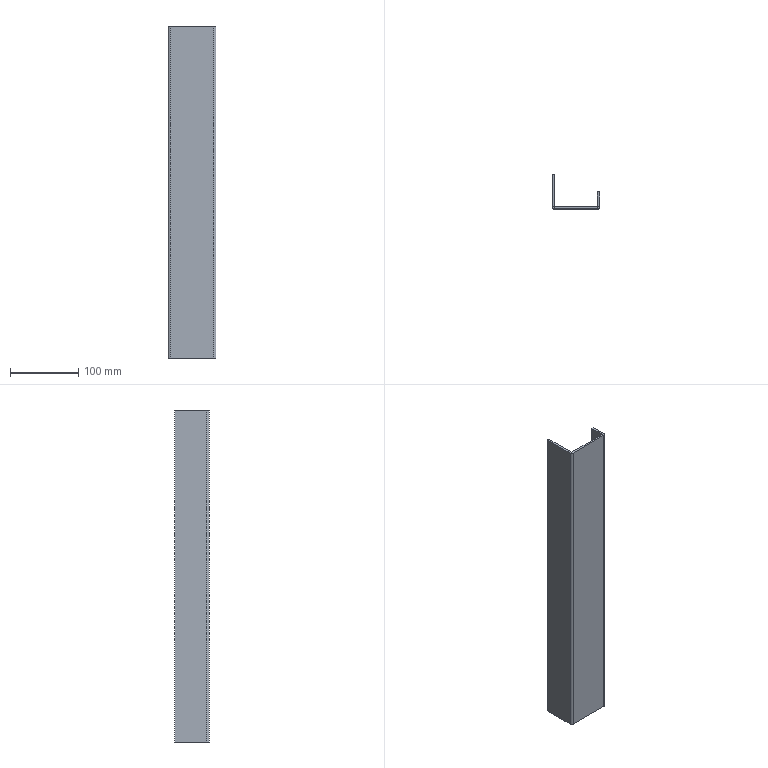Part | SolidWorks | 1 solid | 22 faces | box 69.995 x 50 x 485 mm | volume 200160 mm3 | plane 18 | cylinder 4 | commonest cylinder face diameters 0.2 x2 6.2 x2
STEP:
#1=CARTESIAN_POINT('',(31.895,-3.,-242.5));
#2=VERTEX_POINT('',#1);
#3=CARTESIAN_POINT('',(31.895,-3.,242.5));
#4=VERTEX_POINT('',#3);
#5=CARTESIAN_POINT('',(31.895,-3.,-242.5));
#6=DIRECTION('',(0.,0.,1.));
#7=VECTOR('',#6,1000.);
#8=LINE('',#5,#7);
#9=EDGE_CURVE('',#2,#4,#8,.T.);
#10=ORIENTED_EDGE('',*,*,#9,.T.);
#11=CARTESIAN_POINT('',(-31.9,-3.,242.5));
#12=VERTEX_POINT('',#11);
#13=CARTESIAN_POINT('',(35.,-3.,242.5));
#14=DIRECTION('',(1.,0.,0.));
#15=VECTOR('',#14,1000.);
#16=LINE('',#13,#15);
#17=EDGE_CURVE('',#12,#4,#16,.T.);
#18=ORIENTED_EDGE('',*,*,#17,.F.);
#19=CARTESIAN_POINT('',(-31.9,-3.,-242.5));
#20=VERTEX_POINT('',#19);
#21=CARTESIAN_POINT('',(-31.9,-3.,242.5));
#22=DIRECTION('',(0.,0.,-1.));
#23=VECTOR('',#22,1000.);
#24=LINE('',#21,#23);
#25=EDGE_CURVE('',#12,#20,#24,.T.);
#26=ORIENTED_EDGE('',*,*,#25,.T.);
#27=CARTESIAN_POINT('',(35.,-3.,-242.5));
#28=DIRECTION('',(-1.,0.,0.));
#29=VECTOR('',#28,1000.);
#30=LINE('',#27,#29);
#31=EDGE_CURVE('',#2,#20,#30,.T.);
#32=ORIENTED_EDGE('',*,*,#31,.F.);
#33=EDGE_LOOP('',(#10,#18,#26,#32));
#34=FACE_OUTER_BOUND('',#33,.T.);
#35=CARTESIAN_POINT('',(0.,-3.,0.));
#36=DIRECTION('',(0.,1.,0.));
#37=DIRECTION('',(0.,0.,1.));
#38=AXIS2_PLACEMENT_3D('',#35,#36,#37);
#39=PLANE('',#38);
#40=ADVANCED_FACE('',(#34),#39,.F.);
#41=CARTESIAN_POINT('',(-31.9,0.,242.5));
#42=VERTEX_POINT('',#41);
#43=CARTESIAN_POINT('',(31.895,0.,242.5));
#44=VERTEX_POINT('',#43);
#45=CARTESIAN_POINT('',(35.,0.,242.5));
#46=DIRECTION('',(1.,0.,0.));
#47=VECTOR('',#46,1000.);
#48=LINE('',#45,#47);
#49=EDGE_CURVE('',#42,#44,#48,.T.);
#50=ORIENTED_EDGE('',*,*,#49,.T.);
#51=CARTESIAN_POINT('',(31.895,0.,-242.5));
#52=VERTEX_POINT('',#51);
#53=CARTESIAN_POINT('',(31.895,0.,-242.5));
#54=DIRECTION('',(0.,0.,1.));
#55=VECTOR('',#54,1000.);
#56=LINE('',#53,#55);
#57=EDGE_CURVE('',#52,#44,#56,.T.);
#58=ORIENTED_EDGE('',*,*,#57,.F.);
#59=CARTESIAN_POINT('',(-31.9,0.,-242.5));
#60=VERTEX_POINT('',#59);
#61=CARTESIAN_POINT('',(35.,0.,-242.5));
#62=DIRECTION('',(-1.,0.,0.));
#63=VECTOR('',#62,1000.);
#64=LINE('',#61,#63);
#65=EDGE_CURVE('',#52,#60,#64,.T.);
#66=ORIENTED_EDGE('',*,*,#65,.T.);
#67=CARTESIAN_POINT('',(-31.9,0.,242.5));
#68=DIRECTION('',(0.,0.,-1.));
#69=VECTOR('',#68,1000.);
#70=LINE('',#67,#69);
#71=EDGE_CURVE('',#42,#60,#70,.T.);
#72=ORIENTED_EDGE('',*,*,#71,.F.);
#73=EDGE_LOOP('',(#50,#58,#66,#72));
#74=FACE_OUTER_BOUND('',#73,.T.);
#75=CARTESIAN_POINT('',(0.,0.,0.));
#76=DIRECTION('',(0.,1.,0.));
#77=DIRECTION('',(0.,0.,1.));
#78=AXIS2_PLACEMENT_3D('',#75,#76,#77);
#79=PLANE('',#78);
#80=ADVANCED_FACE('',(#74),#79,.T.);
#81=ORIENTED_EDGE('',*,*,#65,.F.);
#82=CARTESIAN_POINT('',(31.895,0.,-242.5));
#83=DIRECTION('',(0.,-1.,0.));
#84=VECTOR('',#83,1000.);
#85=LINE('',#82,#84);
#86=EDGE_CURVE('',#52,#2,#85,.T.);
#87=ORIENTED_EDGE('',*,*,#86,.T.);
#88=ORIENTED_EDGE('',*,*,#31,.T.);
#89=CARTESIAN_POINT('',(-31.9,0.,-242.5));
#90=DIRECTION('',(0.,-1.,0.));
#91=VECTOR('',#90,1000.);
#92=LINE('',#89,#91);
#93=EDGE_CURVE('',#60,#20,#92,.T.);
#94=ORIENTED_EDGE('',*,*,#93,.F.);
#95=EDGE_LOOP('',(#81,#87,#88,#94));
#96=FACE_OUTER_BOUND('',#95,.T.);
#97=CARTESIAN_POINT('',(35.,-3.,-242.5));
#98=DIRECTION('',(0.,0.,-1.));
#99=DIRECTION('',(-1.,0.,0.));
#100=AXIS2_PLACEMENT_3D('',#97,#98,#99);
#101=PLANE('',#100);
#102=ADVANCED_FACE('',(#96),#101,.T.);
#103=CARTESIAN_POINT('',(31.895,0.,242.5));
#104=DIRECTION('',(0.,-1.,0.));
#105=VECTOR('',#104,1000.);
#106=LINE('',#103,#105);
#107=EDGE_CURVE('',#44,#4,#106,.T.);
#108=ORIENTED_EDGE('',*,*,#107,.F.);
#109=ORIENTED_EDGE('',*,*,#49,.F.);
#110=CARTESIAN_POINT('',(-31.9,0.,242.5));
#111=DIRECTION('',(0.,-1.,0.));
#112=VECTOR('',#111,1000.);
#113=LINE('',#110,#112);
#114=EDGE_CURVE('',#42,#12,#113,.T.);
#115=ORIENTED_EDGE('',*,*,#114,.T.);
#116=ORIENTED_EDGE('',*,*,#17,.T.);
#117=EDGE_LOOP('',(#108,#109,#115,#116));
#118=FACE_OUTER_BOUND('',#117,.T.);
#119=CARTESIAN_POINT('',(35.,-3.,242.5));
#120=DIRECTION('',(0.,0.,1.));
#121=DIRECTION('',(1.,0.,0.));
#122=AXIS2_PLACEMENT_3D('',#119,#120,#121);
#123=PLANE('',#122);
#124=ADVANCED_FACE('',(#118),#123,.T.);
#125=CARTESIAN_POINT('',(-32.,0.1,-242.5));
#126=VERTEX_POINT('',#125);
#127=CARTESIAN_POINT('',(-35.,0.1,-242.5));
#128=VERTEX_POINT('',#127);
#129=CARTESIAN_POINT('',(-35.,0.1,-242.5));
#130=DIRECTION('',(-1.,0.,0.));
#131=VECTOR('',#130,1000.);
#132=LINE('',#129,#131);
#133=EDGE_CURVE('',#126,#128,#132,.T.);
#134=ORIENTED_EDGE('',*,*,#133,.F.);
#135=CARTESIAN_POINT('',(-31.9,0.1,-242.5));
#136=DIRECTION('',(0.,0.,-1.));
#137=DIRECTION('',(1.,0.,0.));
#138=AXIS2_PLACEMENT_3D('',#135,#136,#137);
#139=CIRCLE('',#138,0.1);
#140=EDGE_CURVE('',#60,#126,#139,.T.);
#141=ORIENTED_EDGE('',*,*,#140,.F.);
#142=ORIENTED_EDGE('',*,*,#93,.T.);
#143=CARTESIAN_POINT('',(-31.9,0.1,-242.5));
#144=DIRECTION('',(0.,0.,-1.));
#145=DIRECTION('',(1.,0.,0.));
#146=AXIS2_PLACEMENT_3D('',#143,#144,#145);
#147=CIRCLE('',#146,3.1);
#148=EDGE_CURVE('',#20,#128,#147,.T.);
#149=ORIENTED_EDGE('',*,*,#148,.T.);
#150=EDGE_LOOP('',(#134,#141,#142,#149));
#151=FACE_OUTER_BOUND('',#150,.T.);
#152=CARTESIAN_POINT('',(-31.9,0.1,-242.5));
#153=DIRECTION('',(0.,0.,-1.));
#154=DIRECTION('',(-1.,0.,0.));
#155=AXIS2_PLACEMENT_3D('',#152,#153,#154);
#156=PLANE('',#155);
#157=ADVANCED_FACE('',(#151),#156,.T.);
#158=CARTESIAN_POINT('',(-32.,0.1,242.5));
#159=VERTEX_POINT('',#158);
#160=CARTESIAN_POINT('',(-31.9,0.1,242.5));
#161=DIRECTION('',(0.,0.,1.));
#162=DIRECTION('',(1.,0.,0.));
#163=AXIS2_PLACEMENT_3D('',#160,#161,#162);
#164=CIRCLE('',#163,0.1);
#165=EDGE_CURVE('',#159,#42,#164,.T.);
#166=ORIENTED_EDGE('',*,*,#165,.F.);
#167=CARTESIAN_POINT('',(-35.,0.1,242.5));
#168=VERTEX_POINT('',#167);
#169=CARTESIAN_POINT('',(-32.,0.1,242.5));
#170=DIRECTION('',(-1.,0.,0.));
#171=VECTOR('',#170,1000.);
#172=LINE('',#169,#171);
#173=EDGE_CURVE('',#159,#168,#172,.T.);
#174=ORIENTED_EDGE('',*,*,#173,.T.);
#175=CARTESIAN_POINT('',(-31.9,0.1,242.5));
#176=DIRECTION('',(0.,0.,1.));
#177=DIRECTION('',(1.,0.,0.));
#178=AXIS2_PLACEMENT_3D('',#175,#176,#177);
#179=CIRCLE('',#178,3.1);
#180=EDGE_CURVE('',#168,#12,#179,.T.);
#181=ORIENTED_EDGE('',*,*,#180,.T.);
#182=ORIENTED_EDGE('',*,*,#114,.F.);
#183=EDGE_LOOP('',(#166,#174,#181,#182));
#184=FACE_OUTER_BOUND('',#183,.T.);
#185=CARTESIAN_POINT('',(-31.9,0.1,242.5));
#186=DIRECTION('',(0.,0.,-1.));
#187=DIRECTION('',(-1.,0.,0.));
#188=AXIS2_PLACEMENT_3D('',#185,#186,#187);
#189=PLANE('',#188);
#190=ADVANCED_FACE('',(#184),#189,.F.);
#191=ORIENTED_EDGE('',*,*,#25,.F.);
#192=ORIENTED_EDGE('',*,*,#180,.F.);
#193=CARTESIAN_POINT('',(-35.,0.1,-242.5));
#194=DIRECTION('',(0.,0.,-1.));
#195=VECTOR('',#194,1000.);
#196=LINE('',#193,#195);
#197=EDGE_CURVE('',#168,#128,#196,.T.);
#198=ORIENTED_EDGE('',*,*,#197,.T.);
#199=ORIENTED_EDGE('',*,*,#148,.F.);
#200=EDGE_LOOP('',(#191,#192,#198,#199));
#201=FACE_OUTER_BOUND('',#200,.T.);
#202=CARTESIAN_POINT('',(-31.9,0.1,242.5));
#203=DIRECTION('',(0.,0.,1.));
#204=DIRECTION('',(-1.,0.,0.));
#205=AXIS2_PLACEMENT_3D('',#202,#203,#204);
#206=CYLINDRICAL_SURFACE('',#205,3.1);
#207=ADVANCED_FACE('',(#201),#206,.T.);
#208=ORIENTED_EDGE('',*,*,#71,.T.);
#209=ORIENTED_EDGE('',*,*,#140,.T.);
#210=CARTESIAN_POINT('',(-32.,0.1,-242.5));
#211=DIRECTION('',(0.,0.,1.));
#212=VECTOR('',#211,1000.);
#213=LINE('',#210,#212);
#214=EDGE_CURVE('',#126,#159,#213,.T.);
#215=ORIENTED_EDGE('',*,*,#214,.T.);
#216=ORIENTED_EDGE('',*,*,#165,.T.);
#217=EDGE_LOOP('',(#208,#209,#215,#216));
#218=FACE_OUTER_BOUND('',#217,.T.);
#219=CARTESIAN_POINT('',(-31.9,0.1,242.5));
#220=DIRECTION('',(0.,0.,1.));
#221=DIRECTION('',(-1.,0.,0.));
#222=AXIS2_PLACEMENT_3D('',#219,#220,#221);
#223=CYLINDRICAL_SURFACE('',#222,0.1);
#224=ADVANCED_FACE('',(#218),#223,.F.);
#225=ORIENTED_EDGE('',*,*,#133,.T.);
#226=CARTESIAN_POINT('',(-35.,47.,-242.5));
#227=VERTEX_POINT('',#226);
#228=CARTESIAN_POINT('',(-35.,0.,-242.5));
#229=DIRECTION('',(0.,-1.,0.));
#230=VECTOR('',#229,1000.);
#231=LINE('',#228,#230);
#232=EDGE_CURVE('',#227,#128,#231,.T.);
#233=ORIENTED_EDGE('',*,*,#232,.F.);
#234=CARTESIAN_POINT('',(-32.,47.,-242.5));
#235=VERTEX_POINT('',#234);
#236=CARTESIAN_POINT('',(-35.,47.,-242.5));
#237=DIRECTION('',(1.,0.,0.));
#238=VECTOR('',#237,1000.);
#239=LINE('',#236,#238);
#240=EDGE_CURVE('',#227,#235,#239,.T.);
#241=ORIENTED_EDGE('',*,*,#240,.T.);
#242=CARTESIAN_POINT('',(-32.,0.,-242.5));
#243=DIRECTION('',(0.,-1.,0.));
#244=VECTOR('',#243,1000.);
#245=LINE('',#242,#244);
#246=EDGE_CURVE('',#235,#126,#245,.T.);
#247=ORIENTED_EDGE('',*,*,#246,.T.);
#248=EDGE_LOOP('',(#225,#233,#241,#247));
#249=FACE_OUTER_BOUND('',#248,.T.);
#250=CARTESIAN_POINT('',(-35.,0.,-242.5));
#251=DIRECTION('',(0.,0.,1.));
#252=DIRECTION('',(1.,0.,0.));
#253=AXIS2_PLACEMENT_3D('',#250,#251,#252);
#254=PLANE('',#253);
#255=ADVANCED_FACE('',(#249),#254,.F.);
#256=ORIENTED_EDGE('',*,*,#173,.F.);
#257=CARTESIAN_POINT('',(-32.,47.,242.5));
#258=VERTEX_POINT('',#257);
#259=CARTESIAN_POINT('',(-32.,47.,242.5));
#260=DIRECTION('',(0.,1.,0.));
#261=VECTOR('',#260,1000.);
#262=LINE('',#259,#261);
#263=EDGE_CURVE('',#159,#258,#262,.T.);
#264=ORIENTED_EDGE('',*,*,#263,.T.);
#265=CARTESIAN_POINT('',(-35.,47.,242.5));
#266=VERTEX_POINT('',#265);
#267=CARTESIAN_POINT('',(-35.,47.,242.5));
#268=DIRECTION('',(1.,0.,0.));
#269=VECTOR('',#268,1000.);
#270=LINE('',#267,#269);
#271=EDGE_CURVE('',#266,#258,#270,.T.);
#272=ORIENTED_EDGE('',*,*,#271,.F.);
#273=CARTESIAN_POINT('',(-35.,0.,242.5));
#274=DIRECTION('',(0.,1.,0.));
#275=VECTOR('',#274,1000.);
#276=LINE('',#273,#275);
#277=EDGE_CURVE('',#168,#266,#276,.T.);
#278=ORIENTED_EDGE('',*,*,#277,.F.);
#279=EDGE_LOOP('',(#256,#264,#272,#278));
#280=FACE_OUTER_BOUND('',#279,.T.);
#281=CARTESIAN_POINT('',(-35.,47.,242.5));
#282=DIRECTION('',(0.,0.,-1.));
#283=DIRECTION('',(-1.,0.,0.));
#284=AXIS2_PLACEMENT_3D('',#281,#282,#283);
#285=PLANE('',#284);
#286=ADVANCED_FACE('',(#280),#285,.F.);
#287=ORIENTED_EDGE('',*,*,#197,.F.);
#288=ORIENTED_EDGE('',*,*,#277,.T.);
#289=CARTESIAN_POINT('',(-35.,47.,0.));
#290=DIRECTION('',(0.,0.,-1.));
#291=VECTOR('',#290,1000.);
#292=LINE('',#289,#291);
#293=EDGE_CURVE('',#266,#227,#292,.T.);
#294=ORIENTED_EDGE('',*,*,#293,.T.);
#295=ORIENTED_EDGE('',*,*,#232,.T.);
#296=EDGE_LOOP('',(#287,#288,#294,#295));
#297=FACE_OUTER_BOUND('',#296,.T.);
#298=CARTESIAN_POINT('',(-35.,0.,0.));
#299=DIRECTION('',(1.,0.,0.));
#300=DIRECTION('',(0.,1.,0.));
#301=AXIS2_PLACEMENT_3D('',#298,#299,#300);
#302=PLANE('',#301);
#303=ADVANCED_FACE('',(#297),#302,.F.);
#304=ORIENTED_EDGE('',*,*,#263,.F.);
#305=ORIENTED_EDGE('',*,*,#214,.F.);
#306=ORIENTED_EDGE('',*,*,#246,.F.);
#307=CARTESIAN_POINT('',(-32.,47.,-242.5));
#308=DIRECTION('',(0.,0.,-1.));
#309=VECTOR('',#308,1000.);
#310=LINE('',#307,#309);
#311=EDGE_CURVE('',#258,#235,#310,.T.);
#312=ORIENTED_EDGE('',*,*,#311,.F.);
#313=EDGE_LOOP('',(#304,#305,#306,#312));
#314=FACE_OUTER_BOUND('',#313,.T.);
#315=CARTESIAN_POINT('',(-32.,0.,0.));
#316=DIRECTION('',(1.,0.,0.));
#317=DIRECTION('',(0.,1.,0.));
#318=AXIS2_PLACEMENT_3D('',#315,#316,#317);
#319=PLANE('',#318);
#320=ADVANCED_FACE('',(#314),#319,.T.);
#321=ORIENTED_EDGE('',*,*,#311,.T.);
#322=ORIENTED_EDGE('',*,*,#240,.F.);
#323=ORIENTED_EDGE('',*,*,#293,.F.);
#324=ORIENTED_EDGE('',*,*,#271,.T.);
#325=EDGE_LOOP('',(#321,#322,#323,#324));
#326=FACE_OUTER_BOUND('',#325,.T.);
#327=CARTESIAN_POINT('',(-35.,47.,-242.5));
#328=DIRECTION('',(0.,-1.,0.));
#329=DIRECTION('',(1.,0.,0.));
#330=AXIS2_PLACEMENT_3D('',#327,#328,#329);
#331=PLANE('',#330);
#332=ADVANCED_FACE('',(#326),#331,.F.);
#333=CARTESIAN_POINT('',(31.995,0.1035,242.5));
#334=VERTEX_POINT('',#333);
#335=CARTESIAN_POINT('',(34.993,0.2082,242.5));
#336=VERTEX_POINT('',#335);
#337=CARTESIAN_POINT('',(34.993,0.2082,242.5));
#338=DIRECTION('',(0.9994,0.0349,0.));
#339=VECTOR('',#338,1000.);
#340=LINE('',#337,#339);
#341=EDGE_CURVE('',#334,#336,#340,.T.);
#342=ORIENTED_EDGE('',*,*,#341,.F.);
#343=CARTESIAN_POINT('',(31.895,0.1,242.5));
#344=DIRECTION('',(0.,0.,1.));
#345=DIRECTION('',(-1.,0.,0.));
#346=AXIS2_PLACEMENT_3D('',#343,#344,#345);
#347=CIRCLE('',#346,0.1);
#348=EDGE_CURVE('',#44,#334,#347,.T.);
#349=ORIENTED_EDGE('',*,*,#348,.F.);
#350=ORIENTED_EDGE('',*,*,#107,.T.);
#351=CARTESIAN_POINT('',(31.895,0.1,242.5));
#352=DIRECTION('',(0.,0.,1.));
#353=DIRECTION('',(-1.,0.,0.));
#354=AXIS2_PLACEMENT_3D('',#351,#352,#353);
#355=CIRCLE('',#354,3.1);
#356=EDGE_CURVE('',#4,#336,#355,.T.);
#357=ORIENTED_EDGE('',*,*,#356,.T.);
#358=EDGE_LOOP('',(#342,#349,#350,#357));
#359=FACE_OUTER_BOUND('',#358,.T.);
#360=CARTESIAN_POINT('',(31.895,0.1,242.5));
#361=DIRECTION('',(0.,0.,1.));
#362=DIRECTION('',(1.,0.,0.));
#363=AXIS2_PLACEMENT_3D('',#360,#361,#362);
#364=PLANE('',#363);
#365=ADVANCED_FACE('',(#359),#364,.T.);
#366=CARTESIAN_POINT('',(31.995,0.1035,-242.5));
#367=VERTEX_POINT('',#366);
#368=CARTESIAN_POINT('',(31.895,0.1,-242.5));
#369=DIRECTION('',(0.,0.,-1.));
#370=DIRECTION('',(-1.,0.,0.));
#371=AXIS2_PLACEMENT_3D('',#368,#369,#370);
#372=CIRCLE('',#371,0.1);
#373=EDGE_CURVE('',#367,#52,#372,.T.);
#374=ORIENTED_EDGE('',*,*,#373,.F.);
#375=CARTESIAN_POINT('',(34.993,0.2082,-242.5));
#376=VERTEX_POINT('',#375);
#377=CARTESIAN_POINT('',(31.995,0.1035,-242.5));
#378=DIRECTION('',(0.9994,0.0349,0.));
#379=VECTOR('',#378,1000.);
#380=LINE('',#377,#379);
#381=EDGE_CURVE('',#367,#376,#380,.T.);
#382=ORIENTED_EDGE('',*,*,#381,.T.);
#383=CARTESIAN_POINT('',(31.895,0.1,-242.5));
#384=DIRECTION('',(0.,0.,-1.));
#385=DIRECTION('',(-1.,0.,0.));
#386=AXIS2_PLACEMENT_3D('',#383,#384,#385);
#387=CIRCLE('',#386,3.1);
#388=EDGE_CURVE('',#376,#2,#387,.T.);
#389=ORIENTED_EDGE('',*,*,#388,.T.);
#390=ORIENTED_EDGE('',*,*,#86,.F.);
#391=EDGE_LOOP('',(#374,#382,#389,#390));
#392=FACE_OUTER_BOUND('',#391,.T.);
#393=CARTESIAN_POINT('',(31.895,0.1,-242.5));
#394=DIRECTION('',(0.,0.,1.));
#395=DIRECTION('',(1.,0.,0.));
#396=AXIS2_PLACEMENT_3D('',#393,#394,#395);
#397=PLANE('',#396);
#398=ADVANCED_FACE('',(#392),#397,.F.);
#399=ORIENTED_EDGE('',*,*,#9,.F.);
#400=ORIENTED_EDGE('',*,*,#388,.F.);
#401=CARTESIAN_POINT('',(34.993,0.2082,242.5));
#402=DIRECTION('',(0.,0.,1.));
#403=VECTOR('',#402,1000.);
#404=LINE('',#401,#403);
#405=EDGE_CURVE('',#376,#336,#404,.T.);
#406=ORIENTED_EDGE('',*,*,#405,.T.);
#407=ORIENTED_EDGE('',*,*,#356,.F.);
#408=EDGE_LOOP('',(#399,#400,#406,#407));
#409=FACE_OUTER_BOUND('',#408,.T.);
#410=CARTESIAN_POINT('',(31.895,0.1,-242.5));
#411=DIRECTION('',(0.,0.,-1.));
#412=DIRECTION('',(0.9994,0.0349,0.));
#413=AXIS2_PLACEMENT_3D('',#410,#411,#412);
#414=CYLINDRICAL_SURFACE('',#413,3.1);
#415=ADVANCED_FACE('',(#409),#414,.T.);
#416=ORIENTED_EDGE('',*,*,#57,.T.);
#417=ORIENTED_EDGE('',*,*,#348,.T.);
#418=CARTESIAN_POINT('',(31.995,0.1035,242.5));
#419=DIRECTION('',(0.,0.,-1.));
#420=VECTOR('',#419,1000.);
#421=LINE('',#418,#420);
#422=EDGE_CURVE('',#334,#367,#421,.T.);
#423=ORIENTED_EDGE('',*,*,#422,.T.);
#424=ORIENTED_EDGE('',*,*,#373,.T.);
#425=EDGE_LOOP('',(#416,#417,#423,#424));
#426=FACE_OUTER_BOUND('',#425,.T.);
#427=CARTESIAN_POINT('',(31.895,0.1,-242.5));
#428=DIRECTION('',(0.,0.,-1.));
#429=DIRECTION('',(0.9994,0.0349,0.));
#430=AXIS2_PLACEMENT_3D('',#427,#428,#429);
#431=CYLINDRICAL_SURFACE('',#430,0.1);
#432=ADVANCED_FACE('',(#426),#431,.F.);
#433=ORIENTED_EDGE('',*,*,#381,.F.);
#434=CARTESIAN_POINT('',(31.234,21.88,-242.5));
#435=VERTEX_POINT('',#434);
#436=CARTESIAN_POINT('',(31.234,21.88,-242.5));
#437=DIRECTION('',(-0.0349,0.9994,0.));
#438=VECTOR('',#437,1000.);
#439=LINE('',#436,#438);
#440=EDGE_CURVE('',#367,#435,#439,.T.);
#441=ORIENTED_EDGE('',*,*,#440,.T.);
#442=CARTESIAN_POINT('',(34.232,21.985,-242.5));
#443=VERTEX_POINT('',#442);
#444=CARTESIAN_POINT('',(34.232,21.985,-242.5));
#445=DIRECTION('',(-0.9994,-0.0349,0.));
#446=VECTOR('',#445,1000.);
#447=LINE('',#444,#446);
#448=EDGE_CURVE('',#443,#435,#447,.T.);
#449=ORIENTED_EDGE('',*,*,#448,.F.);
#450=CARTESIAN_POINT('',(34.954,1.325,-242.5));
#451=DIRECTION('',(-0.0349,0.9994,0.));
#452=VECTOR('',#451,1000.);
#453=LINE('',#450,#452);
#454=EDGE_CURVE('',#376,#443,#453,.T.);
#455=ORIENTED_EDGE('',*,*,#454,.F.);
#456=EDGE_LOOP('',(#433,#441,#449,#455));
#457=FACE_OUTER_BOUND('',#456,.T.);
#458=CARTESIAN_POINT('',(34.232,21.985,-242.5));
#459=DIRECTION('',(0.,0.,1.));
#460=DIRECTION('',(1.,0.,0.));
#461=AXIS2_PLACEMENT_3D('',#458,#459,#460);
#462=PLANE('',#461);
#463=ADVANCED_FACE('',(#457),#462,.F.);
#464=ORIENTED_EDGE('',*,*,#341,.T.);
#465=CARTESIAN_POINT('',(34.232,21.985,242.5));
#466=VERTEX_POINT('',#465);
#467=CARTESIAN_POINT('',(34.954,1.325,242.5));
#468=DIRECTION('',(0.0349,-0.9994,0.));
#469=VECTOR('',#468,1000.);
#470=LINE('',#467,#469);
#471=EDGE_CURVE('',#466,#336,#470,.T.);
#472=ORIENTED_EDGE('',*,*,#471,.F.);
#473=CARTESIAN_POINT('',(31.234,21.88,242.5));
#474=VERTEX_POINT('',#473);
#475=CARTESIAN_POINT('',(34.232,21.985,242.5));
#476=DIRECTION('',(-0.9994,-0.0349,0.));
#477=VECTOR('',#476,1000.);
#478=LINE('',#475,#477);
#479=EDGE_CURVE('',#466,#474,#478,.T.);
#480=ORIENTED_EDGE('',*,*,#479,.T.);
#481=CARTESIAN_POINT('',(31.998,0.,242.5));
#482=DIRECTION('',(0.0349,-0.9994,0.));
#483=VECTOR('',#482,1000.);
#484=LINE('',#481,#483);
#485=EDGE_CURVE('',#474,#334,#484,.T.);
#486=ORIENTED_EDGE('',*,*,#485,.T.);
#487=EDGE_LOOP('',(#464,#472,#480,#486));
#488=FACE_OUTER_BOUND('',#487,.T.);
#489=CARTESIAN_POINT('',(34.996,0.1047,242.5));
#490=DIRECTION('',(0.,0.,-1.));
#491=DIRECTION('',(-1.,0.,0.));
#492=AXIS2_PLACEMENT_3D('',#489,#490,#491);
#493=PLANE('',#492);
#494=ADVANCED_FACE('',(#488),#493,.F.);
#495=ORIENTED_EDGE('',*,*,#405,.F.);
#496=ORIENTED_EDGE('',*,*,#454,.T.);
#497=CARTESIAN_POINT('',(34.232,21.985,0.));
#498=DIRECTION('',(0.,0.,1.));
#499=VECTOR('',#498,1000.);
#500=LINE('',#497,#499);
#501=EDGE_CURVE('',#443,#466,#500,.T.);
#502=ORIENTED_EDGE('',*,*,#501,.T.);
#503=ORIENTED_EDGE('',*,*,#471,.T.);
#504=EDGE_LOOP('',(#495,#496,#502,#503));
#505=FACE_OUTER_BOUND('',#504,.T.);
#506=CARTESIAN_POINT('',(34.954,1.325,0.));
#507=DIRECTION('',(-0.9994,-0.0349,0.));
#508=DIRECTION('',(0.0349,-0.9994,0.));
#509=AXIS2_PLACEMENT_3D('',#506,#507,#508);
#510=PLANE('',#509);
#511=ADVANCED_FACE('',(#505),#510,.F.);
#512=ORIENTED_EDGE('',*,*,#440,.F.);
#513=ORIENTED_EDGE('',*,*,#422,.F.);
#514=ORIENTED_EDGE('',*,*,#485,.F.);
#515=CARTESIAN_POINT('',(31.234,21.88,242.5));
#516=DIRECTION('',(0.,0.,1.));
#517=VECTOR('',#516,1000.);
#518=LINE('',#515,#517);
#519=EDGE_CURVE('',#435,#474,#518,.T.);
#520=ORIENTED_EDGE('',*,*,#519,.F.);
#521=EDGE_LOOP('',(#512,#513,#514,#520));
#522=FACE_OUTER_BOUND('',#521,.T.);
#523=CARTESIAN_POINT('',(31.956,1.221,0.));
#524=DIRECTION('',(-0.9994,-0.0349,0.));
#525=DIRECTION('',(0.0349,-0.9994,0.));
#526=AXIS2_PLACEMENT_3D('',#523,#524,#525);
#527=PLANE('',#526);
#528=ADVANCED_FACE('',(#522),#527,.T.);
#529=ORIENTED_EDGE('',*,*,#519,.T.);
#530=ORIENTED_EDGE('',*,*,#479,.F.);
#531=ORIENTED_EDGE('',*,*,#501,.F.);
#532=ORIENTED_EDGE('',*,*,#448,.T.);
#533=EDGE_LOOP('',(#529,#530,#531,#532));
#534=FACE_OUTER_BOUND('',#533,.T.);
#535=CARTESIAN_POINT('',(34.232,21.985,242.5));
#536=DIRECTION('',(0.0349,-0.9994,0.));
#537=DIRECTION('',(0.9994,0.0349,0.));
#538=AXIS2_PLACEMENT_3D('',#535,#536,#537);
#539=PLANE('',#538);
#540=ADVANCED_FACE('',(#534),#539,.F.);
#541=CLOSED_SHELL('',(#40,#80,#102,#124,#157,#190,#207,#224,#255,#286,#303,#320,#332,#365,#398,#415,#432,#463,#494,#511,#528,#540));
#542=MANIFOLD_SOLID_BREP('',#541);
#543=CARTESIAN_POINT('',(0.,0.,0.));
#544=DIRECTION('',(0.,0.,1.));
#545=DIRECTION('',(1.,0.,0.));
#546=AXIS2_PLACEMENT_3D('',#543,#544,#545);
#547=(LENGTH_UNIT()NAMED_UNIT(*)SI_UNIT(.MILLI.,.METRE.));
#548=UNCERTAINTY_MEASURE_WITH_UNIT(LENGTH_MEASURE(0.00001),#547,'','');
#549=(NAMED_UNIT(*)PLANE_ANGLE_UNIT()SI_UNIT($,.RADIAN.));
#550=(NAMED_UNIT(*)SI_UNIT($,.STERADIAN.)SOLID_ANGLE_UNIT());
#551=(GEOMETRIC_REPRESENTATION_CONTEXT(3)GLOBAL_UNCERTAINTY_ASSIGNED_CONTEXT((#548))GLOBAL_UNIT_ASSIGNED_CONTEXT((#547,#549,#550))REPRESENTATION_CONTEXT('',''));
#552=ADVANCED_BREP_SHAPE_REPRESENTATION('',(#542,#546),#551);